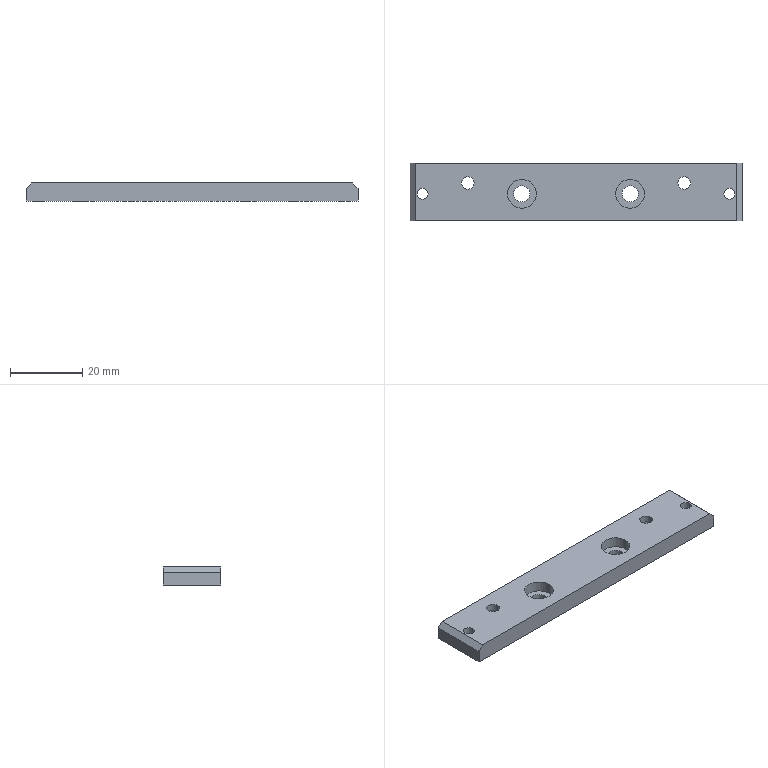NC program | NX | posted with a generic post | part box 92 x 16 x 5 mm
Whole program:
N10 G17 G21 G94 G90
(FLOOR_WALL_COPY , TOOL : D63)
N12 T03 M6
N14 G54
N16 G17 G0 G90 X-80.5 Y0. S6500 M3
N18 G43 Z30. H3
N20 Z5.
N22 G94 G1 Z2. F1500.
N24 X-77.5
N26 X77.5
N28 X80.5
N30 Z5.
N32 G0 Z30.
N34 X-80.5
N36 Z4.
N38 G1 Z1.
N40 X-77.5
N42 X77.5
N44 X80.5
N46 Z4.
N48 G0 Z30.
N50 X-80.5
N52 Z3.
N54 G1 Z0.
N56 X-77.5
N58 X77.5
N60 X80.5
N62 Z3.
N64 G0 Z30.
N66 M5
N68 M2